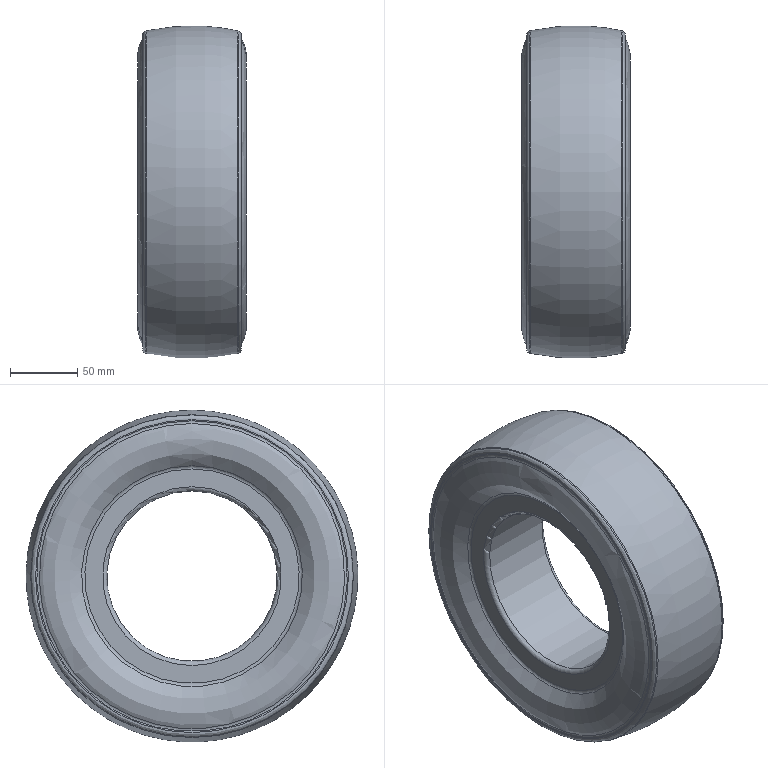Part | NX | features wheel(tire 11x4.00-5) 2 | 1 solid | 36 faces | box 81.098 x 247.904 x 247.904 mm | volume 192340 mm3 | torus 26 | plane 4 | cone 4 | cylinder 2 | commonest cylinder face diameters 127 x1 129.642 x1
STEP:
#1=CARTESIAN_POINT('',(33.738,0.,120.284));
#2=VERTEX_POINT('',#1);
#3=CARTESIAN_POINT('',(33.738,0.,0.));
#4=DIRECTION('',(-1.,0.,0.));
#5=DIRECTION('',(0.,0.,1.));
#6=AXIS2_PLACEMENT_3D('',#3,#4,#5);
#7=CIRCLE('',#6,120.284);
#8=EDGE_CURVE('',#2,#2,#7,.T.);
#9=ORIENTED_EDGE('',*,*,#8,.T.);
#10=EDGE_LOOP('',(#9));
#11=FACE_BOUND('',#10,.T.);
#12=CARTESIAN_POINT('',(-33.738,0.,120.284));
#13=VERTEX_POINT('',#12);
#14=CARTESIAN_POINT('',(-33.738,0.,0.));
#15=DIRECTION('',(-1.,0.,0.));
#16=DIRECTION('',(0.,0.,1.));
#17=AXIS2_PLACEMENT_3D('',#14,#15,#16);
#18=CIRCLE('',#17,120.284);
#19=EDGE_CURVE('',#13,#13,#18,.T.);
#20=ORIENTED_EDGE('',*,*,#19,.F.);
#21=EDGE_LOOP('',(#20));
#22=FACE_BOUND('',#21,.T.);
#23=CARTESIAN_POINT('',(0.,0.,0.));
#24=DIRECTION('',(-1.,0.,0.));
#25=DIRECTION('',(0.,0.,1.));
#26=AXIS2_PLACEMENT_3D('',#23,#24,#25);
#27=DEGENERATE_TOROIDAL_SURFACE('',#26,33.063,157.015,.F.);
#28=ADVANCED_FACE('',(#11,#22),#27,.F.);
#29=CARTESIAN_POINT('',(27.559,0.,63.5));
#30=VERTEX_POINT('',#29);
#31=CARTESIAN_POINT('',(27.559,0.,0.));
#32=DIRECTION('',(-1.,0.,0.));
#33=DIRECTION('',(0.,0.,1.));
#34=AXIS2_PLACEMENT_3D('',#31,#32,#33);
#35=CIRCLE('',#34,63.5);
#36=EDGE_CURVE('',#30,#30,#35,.T.);
#37=ORIENTED_EDGE('',*,*,#36,.F.);
#38=EDGE_LOOP('',(#37));
#39=FACE_BOUND('',#38,.T.);
#40=CARTESIAN_POINT('',(-27.559,0.,63.5));
#41=VERTEX_POINT('',#40);
#42=CARTESIAN_POINT('',(-27.559,0.,0.));
#43=DIRECTION('',(-1.,0.,0.));
#44=DIRECTION('',(0.,0.,1.));
#45=AXIS2_PLACEMENT_3D('',#42,#43,#44);
#46=CIRCLE('',#45,63.5);
#47=EDGE_CURVE('',#41,#41,#46,.T.);
#48=ORIENTED_EDGE('',*,*,#47,.T.);
#49=EDGE_LOOP('',(#48));
#50=FACE_BOUND('',#49,.T.);
#51=CARTESIAN_POINT('',(-55.915,0.,0.));
#52=DIRECTION('',(-1.,0.,0.));
#53=DIRECTION('',(0.,0.,1.));
#54=AXIS2_PLACEMENT_3D('',#51,#52,#53);
#55=CYLINDRICAL_SURFACE('',#54,63.5);
#56=ADVANCED_FACE('',(#39,#50),#55,.F.);
#57=CARTESIAN_POINT('',(30.734,0.,66.675));
#58=VERTEX_POINT('',#57);
#59=CARTESIAN_POINT('',(30.734,0.,0.));
#60=DIRECTION('',(-1.,0.,0.));
#61=DIRECTION('',(0.,0.,1.));
#62=AXIS2_PLACEMENT_3D('',#59,#60,#61);
#63=CIRCLE('',#62,66.675);
#64=EDGE_CURVE('',#58,#58,#63,.T.);
#65=ORIENTED_EDGE('',*,*,#64,.F.);
#66=EDGE_LOOP('',(#65));
#67=FACE_BOUND('',#66,.T.);
#68=ORIENTED_EDGE('',*,*,#36,.T.);
#69=EDGE_LOOP('',(#68));
#70=FACE_BOUND('',#69,.T.);
#71=CARTESIAN_POINT('',(27.559,0.,0.));
#72=DIRECTION('',(-1.,0.,0.));
#73=DIRECTION('',(0.,0.,1.));
#74=AXIS2_PLACEMENT_3D('',#71,#72,#73);
#75=TOROIDAL_SURFACE('',#74,66.675,3.175);
#76=ADVANCED_FACE('',(#67,#70),#75,.T.);
#77=CARTESIAN_POINT('',(30.734,0.,79.901));
#78=VERTEX_POINT('',#77);
#79=CARTESIAN_POINT('',(30.734,0.,0.));
#80=DIRECTION('',(-1.,0.,0.));
#81=DIRECTION('',(0.,0.,1.));
#82=AXIS2_PLACEMENT_3D('',#79,#80,#81);
#83=CIRCLE('',#82,79.901);
#84=EDGE_CURVE('',#78,#78,#83,.T.);
#85=ORIENTED_EDGE('',*,*,#84,.F.);
#86=EDGE_LOOP('',(#85));
#87=FACE_BOUND('',#86,.T.);
#88=ORIENTED_EDGE('',*,*,#64,.T.);
#89=EDGE_LOOP('',(#88));
#90=FACE_BOUND('',#89,.T.);
#91=CARTESIAN_POINT('',(30.734,66.675,0.));
#92=DIRECTION('',(-1.,0.,0.));
#93=DIRECTION('',(0.,0.,1.));
#94=AXIS2_PLACEMENT_3D('',#91,#92,#93);
#95=PLANE('',#94);
#96=ADVANCED_FACE('',(#87,#90),#95,.F.);
#97=CARTESIAN_POINT('',(31.851,0.,82.319));
#98=VERTEX_POINT('',#97);
#99=CARTESIAN_POINT('',(31.851,0.,0.));
#100=DIRECTION('',(-1.,0.,0.));
#101=DIRECTION('',(0.,0.,1.));
#102=AXIS2_PLACEMENT_3D('',#99,#100,#101);
#103=CIRCLE('',#102,82.319);
#104=EDGE_CURVE('',#98,#98,#103,.T.);
#105=ORIENTED_EDGE('',*,*,#104,.F.);
#106=EDGE_LOOP('',(#105));
#107=FACE_BOUND('',#106,.T.);
#108=ORIENTED_EDGE('',*,*,#84,.T.);
#109=EDGE_LOOP('',(#108));
#110=FACE_BOUND('',#109,.T.);
#111=CARTESIAN_POINT('',(33.909,0.,0.));
#112=DIRECTION('',(-1.,0.,0.));
#113=DIRECTION('',(0.,0.,1.));
#114=AXIS2_PLACEMENT_3D('',#111,#112,#113);
#115=TOROIDAL_SURFACE('',#114,79.901,3.175);
#116=ADVANCED_FACE('',(#107,#110),#115,.F.);
#117=CARTESIAN_POINT('',(37.1,0.,113.738));
#118=VERTEX_POINT('',#117);
#119=CARTESIAN_POINT('',(37.1,0.,0.));
#120=DIRECTION('',(-1.,0.,0.));
#121=DIRECTION('',(0.,0.,1.));
#122=AXIS2_PLACEMENT_3D('',#119,#120,#121);
#123=CIRCLE('',#122,113.738);
#124=EDGE_CURVE('',#118,#118,#123,.T.);
#125=ORIENTED_EDGE('',*,*,#124,.F.);
#126=EDGE_LOOP('',(#125));
#127=FACE_BOUND('',#126,.T.);
#128=ORIENTED_EDGE('',*,*,#104,.T.);
#129=EDGE_LOOP('',(#128));
#130=FACE_BOUND('',#129,.T.);
#131=CARTESIAN_POINT('',(15.83,0.,0.));
#132=DIRECTION('',(-1.,0.,0.));
#133=DIRECTION('',(0.,0.,1.));
#134=AXIS2_PLACEMENT_3D('',#131,#132,#133);
#135=TOROIDAL_SURFACE('',#134,101.143,24.719);
#136=ADVANCED_FACE('',(#127,#130),#135,.T.);
#137=CARTESIAN_POINT('',(36.684,0.,115.772));
#138=VERTEX_POINT('',#137);
#139=CARTESIAN_POINT('',(36.684,0.,0.));
#140=DIRECTION('',(-1.,0.,0.));
#141=DIRECTION('',(0.,0.,1.));
#142=AXIS2_PLACEMENT_3D('',#139,#140,#141);
#143=CIRCLE('',#142,115.772);
#144=EDGE_CURVE('',#138,#138,#143,.T.);
#145=ORIENTED_EDGE('',*,*,#144,.F.);
#146=EDGE_LOOP('',(#145));
#147=FACE_BOUND('',#146,.T.);
#148=ORIENTED_EDGE('',*,*,#124,.T.);
#149=EDGE_LOOP('',(#148));
#150=FACE_BOUND('',#149,.T.);
#151=CARTESIAN_POINT('',(39.832,0.,0.));
#152=DIRECTION('',(-1.,0.,0.));
#153=DIRECTION('',(0.,0.,1.));
#154=AXIS2_PLACEMENT_3D('',#151,#152,#153);
#155=TOROIDAL_SURFACE('',#154,115.355,3.175);
#156=ADVANCED_FACE('',(#147,#150),#155,.F.);
#157=CARTESIAN_POINT('',(36.794,0.,116.6));
#158=VERTEX_POINT('',#157);
#159=CARTESIAN_POINT('',(36.794,0.,0.));
#160=DIRECTION('',(-1.,0.,0.));
#161=DIRECTION('',(0.,0.,1.));
#162=AXIS2_PLACEMENT_3D('',#159,#160,#161);
#163=CIRCLE('',#162,116.6);
#164=EDGE_CURVE('',#158,#158,#163,.T.);
#165=ORIENTED_EDGE('',*,*,#164,.F.);
#166=EDGE_LOOP('',(#165));
#167=FACE_BOUND('',#166,.T.);
#168=ORIENTED_EDGE('',*,*,#144,.T.);
#169=EDGE_LOOP('',(#168));
#170=FACE_BOUND('',#169,.T.);
#171=CARTESIAN_POINT('',(36.684,0.,0.));
#172=DIRECTION('',(1.,0.,0.));
#173=DIRECTION('',(0.,0.,-1.));
#174=AXIS2_PLACEMENT_3D('',#171,#172,#173);
#175=CONICAL_SURFACE('',#174,115.772,1.439);
#176=ADVANCED_FACE('',(#167,#170),#175,.F.);
#177=CARTESIAN_POINT('',(34.689,0.,120.016));
#178=VERTEX_POINT('',#177);
#179=CARTESIAN_POINT('',(34.689,0.,0.));
#180=DIRECTION('',(-1.,0.,0.));
#181=DIRECTION('',(0.,0.,1.));
#182=AXIS2_PLACEMENT_3D('',#179,#180,#181);
#183=CIRCLE('',#182,120.016);
#184=EDGE_CURVE('',#178,#178,#183,.T.);
#185=ORIENTED_EDGE('',*,*,#184,.F.);
#186=EDGE_LOOP('',(#185));
#187=FACE_BOUND('',#186,.T.);
#188=ORIENTED_EDGE('',*,*,#164,.T.);
#189=EDGE_LOOP('',(#188));
#190=FACE_BOUND('',#189,.T.);
#191=CARTESIAN_POINT('',(33.646,0.,0.));
#192=DIRECTION('',(-1.,0.,0.));
#193=DIRECTION('',(0.,0.,1.));
#194=AXIS2_PLACEMENT_3D('',#191,#192,#193);
#195=TOROIDAL_SURFACE('',#194,117.017,3.175);
#196=ADVANCED_FACE('',(#187,#190),#195,.T.);
#197=ORIENTED_EDGE('',*,*,#8,.F.);
#198=EDGE_LOOP('',(#197));
#199=FACE_BOUND('',#198,.T.);
#200=ORIENTED_EDGE('',*,*,#184,.T.);
#201=EDGE_LOOP('',(#200));
#202=FACE_BOUND('',#201,.T.);
#203=CARTESIAN_POINT('',(31.937,0.,0.));
#204=DIRECTION('',(-1.,0.,0.));
#205=DIRECTION('',(0.,0.,1.));
#206=AXIS2_PLACEMENT_3D('',#203,#204,#205);
#207=TOROIDAL_SURFACE('',#206,112.098,8.382);
#208=ADVANCED_FACE('',(#199,#202),#207,.T.);
#209=ORIENTED_EDGE('',*,*,#19,.T.);
#210=EDGE_LOOP('',(#209));
#211=FACE_BOUND('',#210,.T.);
#212=CARTESIAN_POINT('',(-34.689,0.,120.016));
#213=VERTEX_POINT('',#212);
#214=CARTESIAN_POINT('',(-34.689,0.,0.));
#215=DIRECTION('',(-1.,0.,0.));
#216=DIRECTION('',(0.,0.,1.));
#217=AXIS2_PLACEMENT_3D('',#214,#215,#216);
#218=CIRCLE('',#217,120.016);
#219=EDGE_CURVE('',#213,#213,#218,.T.);
#220=ORIENTED_EDGE('',*,*,#219,.F.);
#221=EDGE_LOOP('',(#220));
#222=FACE_BOUND('',#221,.T.);
#223=CARTESIAN_POINT('',(-31.937,0.,0.));
#224=DIRECTION('',(1.,0.,0.));
#225=DIRECTION('',(0.,0.,1.));
#226=AXIS2_PLACEMENT_3D('',#223,#224,#225);
#227=TOROIDAL_SURFACE('',#226,112.098,8.382);
#228=ADVANCED_FACE('',(#211,#222),#227,.T.);
#229=ORIENTED_EDGE('',*,*,#219,.T.);
#230=EDGE_LOOP('',(#229));
#231=FACE_BOUND('',#230,.T.);
#232=CARTESIAN_POINT('',(-36.794,0.,116.6));
#233=VERTEX_POINT('',#232);
#234=CARTESIAN_POINT('',(-36.794,0.,0.));
#235=DIRECTION('',(-1.,0.,0.));
#236=DIRECTION('',(0.,0.,1.));
#237=AXIS2_PLACEMENT_3D('',#234,#235,#236);
#238=CIRCLE('',#237,116.6);
#239=EDGE_CURVE('',#233,#233,#238,.T.);
#240=ORIENTED_EDGE('',*,*,#239,.F.);
#241=EDGE_LOOP('',(#240));
#242=FACE_BOUND('',#241,.T.);
#243=CARTESIAN_POINT('',(-33.646,0.,0.));
#244=DIRECTION('',(1.,0.,0.));
#245=DIRECTION('',(0.,0.,1.));
#246=AXIS2_PLACEMENT_3D('',#243,#244,#245);
#247=TOROIDAL_SURFACE('',#246,117.017,3.175);
#248=ADVANCED_FACE('',(#231,#242),#247,.T.);
#249=ORIENTED_EDGE('',*,*,#239,.T.);
#250=EDGE_LOOP('',(#249));
#251=FACE_BOUND('',#250,.T.);
#252=CARTESIAN_POINT('',(-36.684,0.,115.772));
#253=VERTEX_POINT('',#252);
#254=CARTESIAN_POINT('',(-36.684,0.,0.));
#255=DIRECTION('',(-1.,0.,0.));
#256=DIRECTION('',(0.,0.,1.));
#257=AXIS2_PLACEMENT_3D('',#254,#255,#256);
#258=CIRCLE('',#257,115.772);
#259=EDGE_CURVE('',#253,#253,#258,.T.);
#260=ORIENTED_EDGE('',*,*,#259,.F.);
#261=EDGE_LOOP('',(#260));
#262=FACE_BOUND('',#261,.T.);
#263=CARTESIAN_POINT('',(-36.684,0.,0.));
#264=DIRECTION('',(-1.,0.,0.));
#265=DIRECTION('',(0.,0.,-1.));
#266=AXIS2_PLACEMENT_3D('',#263,#264,#265);
#267=CONICAL_SURFACE('',#266,115.772,1.439);
#268=ADVANCED_FACE('',(#251,#262),#267,.F.);
#269=ORIENTED_EDGE('',*,*,#259,.T.);
#270=EDGE_LOOP('',(#269));
#271=FACE_BOUND('',#270,.T.);
#272=CARTESIAN_POINT('',(-37.1,0.,113.738));
#273=VERTEX_POINT('',#272);
#274=CARTESIAN_POINT('',(-37.1,0.,0.));
#275=DIRECTION('',(-1.,0.,0.));
#276=DIRECTION('',(0.,0.,1.));
#277=AXIS2_PLACEMENT_3D('',#274,#275,#276);
#278=CIRCLE('',#277,113.738);
#279=EDGE_CURVE('',#273,#273,#278,.T.);
#280=ORIENTED_EDGE('',*,*,#279,.F.);
#281=EDGE_LOOP('',(#280));
#282=FACE_BOUND('',#281,.T.);
#283=CARTESIAN_POINT('',(-39.832,0.,0.));
#284=DIRECTION('',(1.,0.,0.));
#285=DIRECTION('',(0.,0.,1.));
#286=AXIS2_PLACEMENT_3D('',#283,#284,#285);
#287=TOROIDAL_SURFACE('',#286,115.355,3.175);
#288=ADVANCED_FACE('',(#271,#282),#287,.F.);
#289=ORIENTED_EDGE('',*,*,#279,.T.);
#290=EDGE_LOOP('',(#289));
#291=FACE_BOUND('',#290,.T.);
#292=CARTESIAN_POINT('',(-31.851,0.,82.319));
#293=VERTEX_POINT('',#292);
#294=CARTESIAN_POINT('',(-31.851,0.,0.));
#295=DIRECTION('',(-1.,0.,0.));
#296=DIRECTION('',(0.,0.,1.));
#297=AXIS2_PLACEMENT_3D('',#294,#295,#296);
#298=CIRCLE('',#297,82.319);
#299=EDGE_CURVE('',#293,#293,#298,.T.);
#300=ORIENTED_EDGE('',*,*,#299,.F.);
#301=EDGE_LOOP('',(#300));
#302=FACE_BOUND('',#301,.T.);
#303=CARTESIAN_POINT('',(-15.83,0.,0.));
#304=DIRECTION('',(1.,0.,0.));
#305=DIRECTION('',(0.,0.,1.));
#306=AXIS2_PLACEMENT_3D('',#303,#304,#305);
#307=TOROIDAL_SURFACE('',#306,101.143,24.719);
#308=ADVANCED_FACE('',(#291,#302),#307,.T.);
#309=ORIENTED_EDGE('',*,*,#299,.T.);
#310=EDGE_LOOP('',(#309));
#311=FACE_BOUND('',#310,.T.);
#312=CARTESIAN_POINT('',(-30.734,0.,79.901));
#313=VERTEX_POINT('',#312);
#314=CARTESIAN_POINT('',(-30.734,0.,0.));
#315=DIRECTION('',(-1.,0.,0.));
#316=DIRECTION('',(0.,0.,1.));
#317=AXIS2_PLACEMENT_3D('',#314,#315,#316);
#318=CIRCLE('',#317,79.901);
#319=EDGE_CURVE('',#313,#313,#318,.T.);
#320=ORIENTED_EDGE('',*,*,#319,.F.);
#321=EDGE_LOOP('',(#320));
#322=FACE_BOUND('',#321,.T.);
#323=CARTESIAN_POINT('',(-33.909,0.,0.));
#324=DIRECTION('',(1.,0.,0.));
#325=DIRECTION('',(0.,0.,1.));
#326=AXIS2_PLACEMENT_3D('',#323,#324,#325);
#327=TOROIDAL_SURFACE('',#326,79.901,3.175);
#328=ADVANCED_FACE('',(#311,#322),#327,.F.);
#329=ORIENTED_EDGE('',*,*,#319,.T.);
#330=EDGE_LOOP('',(#329));
#331=FACE_BOUND('',#330,.T.);
#332=CARTESIAN_POINT('',(-30.734,0.,66.675));
#333=VERTEX_POINT('',#332);
#334=CARTESIAN_POINT('',(-30.734,0.,0.));
#335=DIRECTION('',(-1.,0.,0.));
#336=DIRECTION('',(0.,0.,1.));
#337=AXIS2_PLACEMENT_3D('',#334,#335,#336);
#338=CIRCLE('',#337,66.675);
#339=EDGE_CURVE('',#333,#333,#338,.T.);
#340=ORIENTED_EDGE('',*,*,#339,.F.);
#341=EDGE_LOOP('',(#340));
#342=FACE_BOUND('',#341,.T.);
#343=CARTESIAN_POINT('',(-30.734,66.675,0.));
#344=DIRECTION('',(1.,0.,0.));
#345=DIRECTION('',(0.,0.,1.));
#346=AXIS2_PLACEMENT_3D('',#343,#344,#345);
#347=PLANE('',#346);
#348=ADVANCED_FACE('',(#331,#342),#347,.F.);
#349=ORIENTED_EDGE('',*,*,#339,.T.);
#350=EDGE_LOOP('',(#349));
#351=FACE_BOUND('',#350,.T.);
#352=ORIENTED_EDGE('',*,*,#47,.F.);
#353=EDGE_LOOP('',(#352));
#354=FACE_BOUND('',#353,.T.);
#355=CARTESIAN_POINT('',(-27.559,0.,0.));
#356=DIRECTION('',(1.,0.,0.));
#357=DIRECTION('',(0.,0.,1.));
#358=AXIS2_PLACEMENT_3D('',#355,#356,#357);
#359=TOROIDAL_SURFACE('',#358,66.675,3.175);
#360=ADVANCED_FACE('',(#351,#354),#359,.T.);
#361=CLOSED_SHELL('',(#28,#56,#76,#96,#116,#136,#156,#176,#196,#208,#228,#248,#268,#288,#308,#328,#348,#360));
#362=CARTESIAN_POINT('',(-33.454,0.,118.995));
#363=VERTEX_POINT('',#362);
#364=CARTESIAN_POINT('',(-33.454,0.,0.));
#365=DIRECTION('',(-1.,0.,0.));
#366=DIRECTION('',(0.,0.,1.));
#367=AXIS2_PLACEMENT_3D('',#364,#365,#366);
#368=CIRCLE('',#367,118.995);
#369=EDGE_CURVE('',#363,#363,#368,.T.);
#370=ORIENTED_EDGE('',*,*,#369,.F.);
#371=EDGE_LOOP('',(#370));
#372=FACE_BOUND('',#371,.T.);
#373=CARTESIAN_POINT('',(-34.255,0.,118.768));
#374=VERTEX_POINT('',#373);
#375=CARTESIAN_POINT('',(-34.255,0.,0.));
#376=DIRECTION('',(-1.,0.,0.));
#377=DIRECTION('',(0.,0.,1.));
#378=AXIS2_PLACEMENT_3D('',#375,#376,#377);
#379=CIRCLE('',#378,118.768);
#380=EDGE_CURVE('',#374,#374,#379,.T.);
#381=ORIENTED_EDGE('',*,*,#380,.T.);
#382=EDGE_LOOP('',(#381));
#383=FACE_BOUND('',#382,.T.);
#384=CARTESIAN_POINT('',(-31.937,0.,0.));
#385=DIRECTION('',(1.,0.,0.));
#386=DIRECTION('',(0.,0.,1.));
#387=AXIS2_PLACEMENT_3D('',#384,#385,#386);
#388=TOROIDAL_SURFACE('',#387,112.098,7.061);
#389=ADVANCED_FACE('',(#372,#383),#388,.F.);
#390=ORIENTED_EDGE('',*,*,#380,.F.);
#391=EDGE_LOOP('',(#390));
#392=FACE_BOUND('',#391,.T.);
#393=CARTESIAN_POINT('',(-35.484,0.,116.773));
#394=VERTEX_POINT('',#393);
#395=CARTESIAN_POINT('',(-35.484,0.,0.));
#396=DIRECTION('',(-1.,0.,0.));
#397=DIRECTION('',(0.,0.,1.));
#398=AXIS2_PLACEMENT_3D('',#395,#396,#397);
#399=CIRCLE('',#398,116.773);
#400=EDGE_CURVE('',#394,#394,#399,.T.);
#401=ORIENTED_EDGE('',*,*,#400,.T.);
#402=EDGE_LOOP('',(#401));
#403=FACE_BOUND('',#402,.T.);
#404=CARTESIAN_POINT('',(-33.646,0.,0.));
#405=DIRECTION('',(1.,0.,0.));
#406=DIRECTION('',(0.,0.,1.));
#407=AXIS2_PLACEMENT_3D('',#404,#405,#406);
#408=TOROIDAL_SURFACE('',#407,117.017,1.854);
#409=ADVANCED_FACE('',(#392,#403),#408,.F.);
#410=ORIENTED_EDGE('',*,*,#400,.F.);
#411=EDGE_LOOP('',(#410));
#412=FACE_BOUND('',#411,.T.);
#413=CARTESIAN_POINT('',(-35.375,0.,115.946));
#414=VERTEX_POINT('',#413);
#415=CARTESIAN_POINT('',(-35.375,0.,0.));
#416=DIRECTION('',(-1.,0.,0.));
#417=DIRECTION('',(0.,0.,1.));
#418=AXIS2_PLACEMENT_3D('',#415,#416,#417);
#419=CIRCLE('',#418,115.946);
#420=EDGE_CURVE('',#414,#414,#419,.T.);
#421=ORIENTED_EDGE('',*,*,#420,.T.);
#422=EDGE_LOOP('',(#421));
#423=FACE_BOUND('',#422,.T.);
#424=CARTESIAN_POINT('',(-35.375,0.,0.));
#425=DIRECTION('',(-1.,0.,0.));
#426=DIRECTION('',(0.,0.,-1.));
#427=AXIS2_PLACEMENT_3D('',#424,#425,#426);
#428=CONICAL_SURFACE('',#427,115.946,1.439);
#429=ADVANCED_FACE('',(#412,#423),#428,.T.);
#430=ORIENTED_EDGE('',*,*,#420,.F.);
#431=EDGE_LOOP('',(#430));
#432=FACE_BOUND('',#431,.T.);
#433=CARTESIAN_POINT('',(-35.963,0.,113.065));
#434=VERTEX_POINT('',#433);
#435=CARTESIAN_POINT('',(-35.963,0.,0.));
#436=DIRECTION('',(-1.,0.,0.));
#437=DIRECTION('',(0.,0.,1.));
#438=AXIS2_PLACEMENT_3D('',#435,#436,#437);
#439=CIRCLE('',#438,113.065);
#440=EDGE_CURVE('',#434,#434,#439,.T.);
#441=ORIENTED_EDGE('',*,*,#440,.T.);
#442=EDGE_LOOP('',(#441));
#443=FACE_BOUND('',#442,.T.);
#444=CARTESIAN_POINT('',(-39.832,0.,0.));
#445=DIRECTION('',(1.,0.,0.));
#446=DIRECTION('',(0.,0.,1.));
#447=AXIS2_PLACEMENT_3D('',#444,#445,#446);
#448=TOROIDAL_SURFACE('',#447,115.355,4.496);
#449=ADVANCED_FACE('',(#432,#443),#448,.T.);
#450=ORIENTED_EDGE('',*,*,#440,.F.);
#451=EDGE_LOOP('',(#450));
#452=FACE_BOUND('',#451,.T.);
#453=CARTESIAN_POINT('',(-30.995,0.,83.325));
#454=VERTEX_POINT('',#453);
#455=CARTESIAN_POINT('',(-30.995,0.,0.));
#456=DIRECTION('',(-1.,0.,0.));
#457=DIRECTION('',(0.,0.,1.));
#458=AXIS2_PLACEMENT_3D('',#455,#456,#457);
#459=CIRCLE('',#458,83.325);
#460=EDGE_CURVE('',#454,#454,#459,.T.);
#461=ORIENTED_EDGE('',*,*,#460,.T.);
#462=EDGE_LOOP('',(#461));
#463=FACE_BOUND('',#462,.T.);
#464=CARTESIAN_POINT('',(-15.83,0.,0.));
#465=DIRECTION('',(1.,0.,0.));
#466=DIRECTION('',(0.,0.,1.));
#467=AXIS2_PLACEMENT_3D('',#464,#465,#466);
#468=TOROIDAL_SURFACE('',#467,101.143,23.398);
#469=ADVANCED_FACE('',(#452,#463),#468,.F.);
#470=ORIENTED_EDGE('',*,*,#460,.F.);
#471=EDGE_LOOP('',(#470));
#472=FACE_BOUND('',#471,.T.);
#473=CARTESIAN_POINT('',(-29.413,0.,79.901));
#474=VERTEX_POINT('',#473);
#475=CARTESIAN_POINT('',(-29.413,0.,0.));
#476=DIRECTION('',(-1.,0.,0.));
#477=DIRECTION('',(0.,0.,1.));
#478=AXIS2_PLACEMENT_3D('',#475,#476,#477);
#479=CIRCLE('',#478,79.901);
#480=EDGE_CURVE('',#474,#474,#479,.T.);
#481=ORIENTED_EDGE('',*,*,#480,.T.);
#482=EDGE_LOOP('',(#481));
#483=FACE_BOUND('',#482,.T.);
#484=CARTESIAN_POINT('',(-33.909,0.,0.));
#485=DIRECTION('',(1.,0.,0.));
#486=DIRECTION('',(0.,0.,1.));
#487=AXIS2_PLACEMENT_3D('',#484,#485,#486);
#488=TOROIDAL_SURFACE('',#487,79.901,4.496);
#489=ADVANCED_FACE('',(#472,#483),#488,.T.);
#490=ORIENTED_EDGE('',*,*,#480,.F.);
#491=EDGE_LOOP('',(#490));
#492=FACE_BOUND('',#491,.T.);
#493=CARTESIAN_POINT('',(-29.413,0.,66.675));
#494=VERTEX_POINT('',#493);
#495=CARTESIAN_POINT('',(-29.413,0.,0.));
#496=DIRECTION('',(-1.,0.,0.));
#497=DIRECTION('',(0.,0.,1.));
#498=AXIS2_PLACEMENT_3D('',#495,#496,#497);
#499=CIRCLE('',#498,66.675);
#500=EDGE_CURVE('',#494,#494,#499,.T.);
#501=ORIENTED_EDGE('',*,*,#500,.T.);
#502=EDGE_LOOP('',(#501));
#503=FACE_BOUND('',#502,.T.);
#504=CARTESIAN_POINT('',(-29.413,66.675,0.));
#505=DIRECTION('',(1.,0.,0.));
#506=DIRECTION('',(0.,0.,1.));
#507=AXIS2_PLACEMENT_3D('',#504,#505,#506);
#508=PLANE('',#507);
#509=ADVANCED_FACE('',(#492,#503),#508,.T.);
#510=ORIENTED_EDGE('',*,*,#500,.F.);
#511=EDGE_LOOP('',(#510));
#512=FACE_BOUND('',#511,.T.);
#513=CARTESIAN_POINT('',(-27.559,0.,64.821));
#514=VERTEX_POINT('',#513);
#515=CARTESIAN_POINT('',(-27.559,0.,0.));
#516=DIRECTION('',(-1.,0.,0.));
#517=DIRECTION('',(0.,0.,1.));
#518=AXIS2_PLACEMENT_3D('',#515,#516,#517);
#519=CIRCLE('',#518,64.821);
#520=EDGE_CURVE('',#514,#514,#519,.T.);
#521=ORIENTED_EDGE('',*,*,#520,.T.);
#522=EDGE_LOOP('',(#521));
#523=FACE_BOUND('',#522,.T.);
#524=CARTESIAN_POINT('',(-27.559,0.,0.));
#525=DIRECTION('',(1.,0.,0.));
#526=DIRECTION('',(0.,0.,1.));
#527=AXIS2_PLACEMENT_3D('',#524,#525,#526);
#528=TOROIDAL_SURFACE('',#527,66.675,1.854);
#529=ADVANCED_FACE('',(#512,#523),#528,.F.);
#530=CARTESIAN_POINT('',(35.963,0.,113.065));
#531=VERTEX_POINT('',#530);
#532=CARTESIAN_POINT('',(35.963,0.,0.));
#533=DIRECTION('',(-1.,0.,0.));
#534=DIRECTION('',(0.,0.,1.));
#535=AXIS2_PLACEMENT_3D('',#532,#533,#534);
#536=CIRCLE('',#535,113.065);
#537=EDGE_CURVE('',#531,#531,#536,.T.);
#538=ORIENTED_EDGE('',*,*,#537,.T.);
#539=EDGE_LOOP('',(#538));
#540=FACE_BOUND('',#539,.T.);
#541=CARTESIAN_POINT('',(30.995,0.,83.325));
#542=VERTEX_POINT('',#541);
#543=CARTESIAN_POINT('',(30.995,0.,0.));
#544=DIRECTION('',(-1.,0.,0.));
#545=DIRECTION('',(0.,0.,1.));
#546=AXIS2_PLACEMENT_3D('',#543,#544,#545);
#547=CIRCLE('',#546,83.325);
#548=EDGE_CURVE('',#542,#542,#547,.T.);
#549=ORIENTED_EDGE('',*,*,#548,.F.);
#550=EDGE_LOOP('',(#549));
#551=FACE_BOUND('',#550,.T.);
#552=CARTESIAN_POINT('',(15.83,0.,0.));
#553=DIRECTION('',(-1.,0.,0.));
#554=DIRECTION('',(0.,0.,1.));
#555=AXIS2_PLACEMENT_3D('',#552,#553,#554);
#556=TOROIDAL_SURFACE('',#555,101.143,23.398);
#557=ADVANCED_FACE('',(#540,#551),#556,.F.);
#558=ORIENTED_EDGE('',*,*,#548,.T.);
#559=EDGE_LOOP('',(#558));
#560=FACE_BOUND('',#559,.T.);
#561=CARTESIAN_POINT('',(29.413,0.,79.901));
#562=VERTEX_POINT('',#561);
#563=CARTESIAN_POINT('',(29.413,0.,0.));
#564=DIRECTION('',(-1.,0.,0.));
#565=DIRECTION('',(0.,0.,1.));
#566=AXIS2_PLACEMENT_3D('',#563,#564,#565);
#567=CIRCLE('',#566,79.901);
#568=EDGE_CURVE('',#562,#562,#567,.T.);
#569=ORIENTED_EDGE('',*,*,#568,.F.);
#570=EDGE_LOOP('',(#569));
#571=FACE_BOUND('',#570,.T.);
#572=CARTESIAN_POINT('',(33.909,0.,0.));
#573=DIRECTION('',(-1.,0.,0.));
#574=DIRECTION('',(0.,0.,1.));
#575=AXIS2_PLACEMENT_3D('',#572,#573,#574);
#576=TOROIDAL_SURFACE('',#575,79.901,4.496);
#577=ADVANCED_FACE('',(#560,#571),#576,.T.);
#578=ORIENTED_EDGE('',*,*,#568,.T.);
#579=EDGE_LOOP('',(#578));
#580=FACE_BOUND('',#579,.T.);
#581=CARTESIAN_POINT('',(29.413,0.,66.675));
#582=VERTEX_POINT('',#581);
#583=CARTESIAN_POINT('',(29.413,0.,0.));
#584=DIRECTION('',(-1.,0.,0.));
#585=DIRECTION('',(0.,0.,1.));
#586=AXIS2_PLACEMENT_3D('',#583,#584,#585);
#587=CIRCLE('',#586,66.675);
#588=EDGE_CURVE('',#582,#582,#587,.T.);
#589=ORIENTED_EDGE('',*,*,#588,.F.);
#590=EDGE_LOOP('',(#589));
#591=FACE_BOUND('',#590,.T.);
#592=CARTESIAN_POINT('',(29.413,66.675,0.));
#593=DIRECTION('',(-1.,0.,0.));
#594=DIRECTION('',(0.,0.,1.));
#595=AXIS2_PLACEMENT_3D('',#592,#593,#594);
#596=PLANE('',#595);
#597=ADVANCED_FACE('',(#580,#591),#596,.T.);
#598=ORIENTED_EDGE('',*,*,#588,.T.);
#599=EDGE_LOOP('',(#598));
#600=FACE_BOUND('',#599,.T.);
#601=CARTESIAN_POINT('',(27.559,0.,64.821));
#602=VERTEX_POINT('',#601);
#603=CARTESIAN_POINT('',(27.559,0.,0.));
#604=DIRECTION('',(-1.,0.,0.));
#605=DIRECTION('',(0.,0.,1.));
#606=AXIS2_PLACEMENT_3D('',#603,#604,#605);
#607=CIRCLE('',#606,64.821);
#608=EDGE_CURVE('',#602,#602,#607,.T.);
#609=ORIENTED_EDGE('',*,*,#608,.F.);
#610=EDGE_LOOP('',(#609));
#611=FACE_BOUND('',#610,.T.);
#612=CARTESIAN_POINT('',(27.559,0.,0.));
#613=DIRECTION('',(-1.,0.,0.));
#614=DIRECTION('',(0.,0.,1.));
#615=AXIS2_PLACEMENT_3D('',#612,#613,#614);
#616=TOROIDAL_SURFACE('',#615,66.675,1.854);
#617=ADVANCED_FACE('',(#600,#611),#616,.F.);
#618=ORIENTED_EDGE('',*,*,#608,.T.);
#619=EDGE_LOOP('',(#618));
#620=FACE_BOUND('',#619,.T.);
#621=ORIENTED_EDGE('',*,*,#520,.F.);
#622=EDGE_LOOP('',(#621));
#623=FACE_BOUND('',#622,.T.);
#624=CARTESIAN_POINT('',(-55.915,0.,0.));
#625=DIRECTION('',(-1.,0.,0.));
#626=DIRECTION('',(0.,0.,1.));
#627=AXIS2_PLACEMENT_3D('',#624,#625,#626);
#628=CYLINDRICAL_SURFACE('',#627,64.821);
#629=ADVANCED_FACE('',(#620,#623),#628,.T.);
#630=CARTESIAN_POINT('',(35.375,0.,115.946));
#631=VERTEX_POINT('',#630);
#632=CARTESIAN_POINT('',(35.375,0.,0.));
#633=DIRECTION('',(-1.,0.,0.));
#634=DIRECTION('',(0.,0.,1.));
#635=AXIS2_PLACEMENT_3D('',#632,#633,#634);
#636=CIRCLE('',#635,115.946);
#637=EDGE_CURVE('',#631,#631,#636,.T.);
#638=ORIENTED_EDGE('',*,*,#637,.T.);
#639=EDGE_LOOP('',(#638));
#640=FACE_BOUND('',#639,.T.);
#641=ORIENTED_EDGE('',*,*,#537,.F.);
#642=EDGE_LOOP('',(#641));
#643=FACE_BOUND('',#642,.T.);
#644=CARTESIAN_POINT('',(39.832,0.,0.));
#645=DIRECTION('',(-1.,0.,0.));
#646=DIRECTION('',(0.,0.,1.));
#647=AXIS2_PLACEMENT_3D('',#644,#645,#646);
#648=TOROIDAL_SURFACE('',#647,115.355,4.496);
#649=ADVANCED_FACE('',(#640,#643),#648,.T.);
#650=CARTESIAN_POINT('',(35.484,0.,116.773));
#651=VERTEX_POINT('',#650);
#652=CARTESIAN_POINT('',(35.484,0.,0.));
#653=DIRECTION('',(-1.,0.,0.));
#654=DIRECTION('',(0.,0.,1.));
#655=AXIS2_PLACEMENT_3D('',#652,#653,#654);
#656=CIRCLE('',#655,116.773);
#657=EDGE_CURVE('',#651,#651,#656,.T.);
#658=ORIENTED_EDGE('',*,*,#657,.T.);
#659=EDGE_LOOP('',(#658));
#660=FACE_BOUND('',#659,.T.);
#661=ORIENTED_EDGE('',*,*,#637,.F.);
#662=EDGE_LOOP('',(#661));
#663=FACE_BOUND('',#662,.T.);
#664=CARTESIAN_POINT('',(35.375,0.,0.));
#665=DIRECTION('',(1.,0.,0.));
#666=DIRECTION('',(0.,0.,-1.));
#667=AXIS2_PLACEMENT_3D('',#664,#665,#666);
#668=CONICAL_SURFACE('',#667,115.946,1.439);
#669=ADVANCED_FACE('',(#660,#663),#668,.T.);
#670=CARTESIAN_POINT('',(34.255,0.,118.768));
#671=VERTEX_POINT('',#670);
#672=CARTESIAN_POINT('',(34.255,0.,0.));
#673=DIRECTION('',(-1.,0.,0.));
#674=DIRECTION('',(0.,0.,1.));
#675=AXIS2_PLACEMENT_3D('',#672,#673,#674);
#676=CIRCLE('',#675,118.768);
#677=EDGE_CURVE('',#671,#671,#676,.T.);
#678=ORIENTED_EDGE('',*,*,#677,.T.);
#679=EDGE_LOOP('',(#678));
#680=FACE_BOUND('',#679,.T.);
#681=ORIENTED_EDGE('',*,*,#657,.F.);
#682=EDGE_LOOP('',(#681));
#683=FACE_BOUND('',#682,.T.);
#684=CARTESIAN_POINT('',(33.646,0.,0.));
#685=DIRECTION('',(-1.,0.,0.));
#686=DIRECTION('',(0.,0.,1.));
#687=AXIS2_PLACEMENT_3D('',#684,#685,#686);
#688=TOROIDAL_SURFACE('',#687,117.017,1.854);
#689=ADVANCED_FACE('',(#680,#683),#688,.F.);
#690=CARTESIAN_POINT('',(33.454,0.,118.995));
#691=VERTEX_POINT('',#690);
#692=CARTESIAN_POINT('',(33.454,0.,0.));
#693=DIRECTION('',(-1.,0.,0.));
#694=DIRECTION('',(0.,0.,1.));
#695=AXIS2_PLACEMENT_3D('',#692,#693,#694);
#696=CIRCLE('',#695,118.995);
#697=EDGE_CURVE('',#691,#691,#696,.T.);
#698=ORIENTED_EDGE('',*,*,#697,.T.);
#699=EDGE_LOOP('',(#698));
#700=FACE_BOUND('',#699,.T.);
#701=ORIENTED_EDGE('',*,*,#677,.F.);
#702=EDGE_LOOP('',(#701));
#703=FACE_BOUND('',#702,.T.);
#704=CARTESIAN_POINT('',(31.937,0.,0.));
#705=DIRECTION('',(-1.,0.,0.));
#706=DIRECTION('',(0.,0.,1.));
#707=AXIS2_PLACEMENT_3D('',#704,#705,#706);
#708=TOROIDAL_SURFACE('',#707,112.098,7.061);
#709=ADVANCED_FACE('',(#700,#703),#708,.F.);
#710=ORIENTED_EDGE('',*,*,#697,.F.);
#711=EDGE_LOOP('',(#710));
#712=FACE_BOUND('',#711,.T.);
#713=ORIENTED_EDGE('',*,*,#369,.T.);
#714=EDGE_LOOP('',(#713));
#715=FACE_BOUND('',#714,.T.);
#716=CARTESIAN_POINT('',(0.,0.,0.));
#717=DIRECTION('',(-1.,0.,0.));
#718=DIRECTION('',(0.,0.,1.));
#719=AXIS2_PLACEMENT_3D('',#716,#717,#718);
#720=DEGENERATE_TOROIDAL_SURFACE('',#719,33.063,155.695,.F.);
#721=ADVANCED_FACE('',(#712,#715),#720,.T.);
#722=CLOSED_SHELL('',(#389,#409,#429,#449,#469,#489,#509,#529,#557,#577,#597,#617,#629,#649,#669,#689,#709,#721));
#723=ORIENTED_CLOSED_SHELL('',*,#722,.F.);
#724=BREP_WITH_VOIDS('',#361,(#723));
#725=(LENGTH_UNIT()NAMED_UNIT(*)SI_UNIT(.MILLI.,.METRE.));
#726=UNCERTAINTY_MEASURE_WITH_UNIT(LENGTH_MEASURE(0.00001),#725,'','');
#727=(NAMED_UNIT(*)PLANE_ANGLE_UNIT()SI_UNIT($,.RADIAN.));
#728=(NAMED_UNIT(*)SI_UNIT($,.STERADIAN.)SOLID_ANGLE_UNIT());
#729=(GEOMETRIC_REPRESENTATION_CONTEXT(3)GLOBAL_UNCERTAINTY_ASSIGNED_CONTEXT((#726))GLOBAL_UNIT_ASSIGNED_CONTEXT((#725,#727,#728))REPRESENTATION_CONTEXT('',''));
#730=ADVANCED_BREP_SHAPE_REPRESENTATION('',(#724),#729);